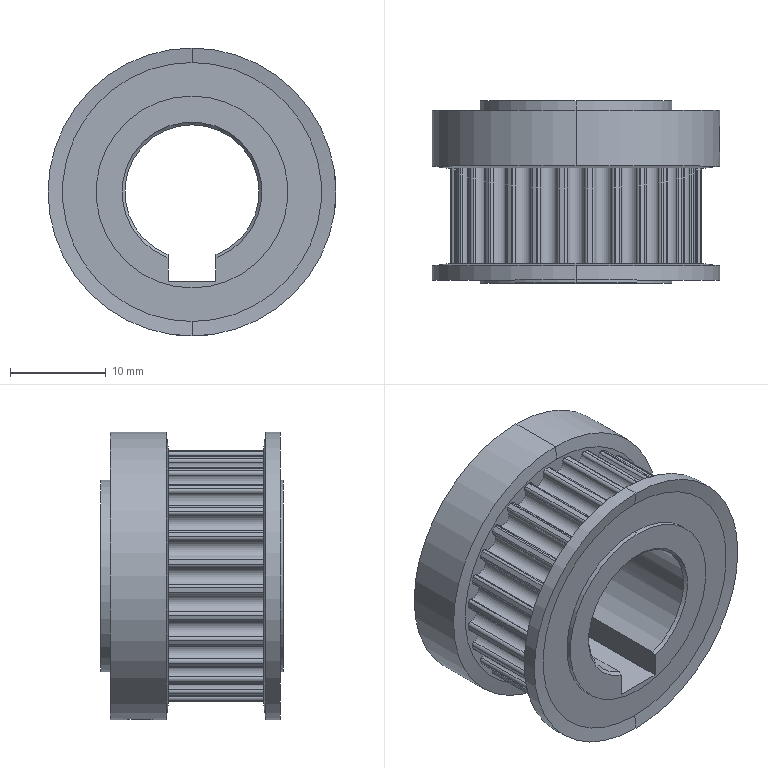Part | STEP file | Timing pulley 28-3M-φ14-19-J | 1 solid | 170 faces | box 30 x 19 x 30 mm | volume 7318 mm3 | cylinder 152 | cone 9 | plane 9 | commonest cylinder face diameters 0.665 x68 1.8 x42 26.22 x28 3.3 x4 20 x4 30 x4